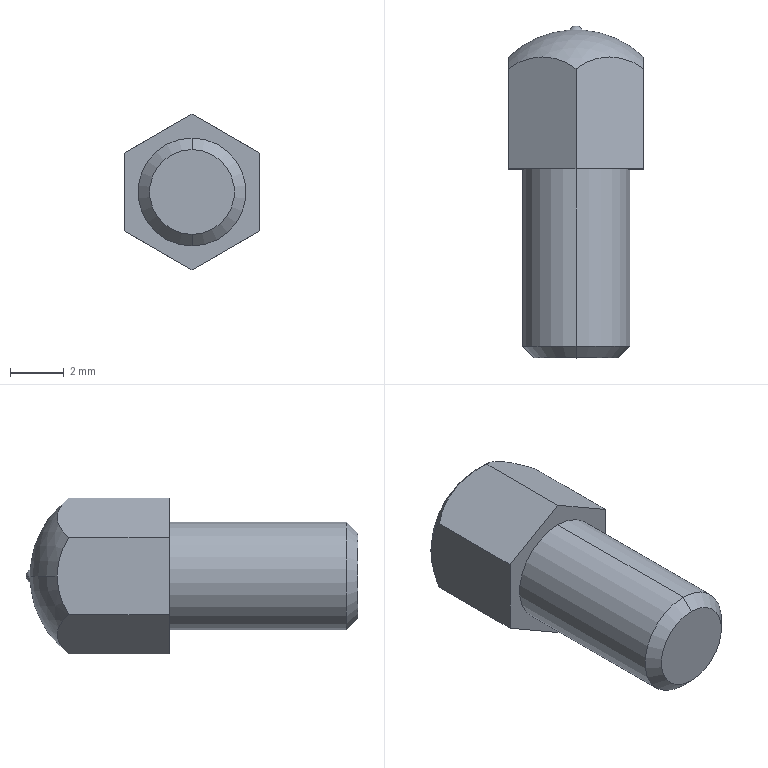Part | STEP file | HG15_34310002 | 1 solid | 16 faces | box 5 x 12.3 x 5.774 mm | volume 186.95 mm3 | plane 8 | sphere 4 | cone 2 | cylinder 2 | commonest cylinder face diameters 4 x2
STEP:
#1=CARTESIAN_POINT('',(0.,0.,0.));
#2=DIRECTION('',(0.,0.,1.));
#3=DIRECTION('',(1.,0.,0.));
#4=AXIS2_PLACEMENT_3D('',#1,#2,#3);
#5=CARTESIAN_POINT('',(-2.5,3.711,-1.443));
#6=VERTEX_POINT('',#5);
#7=CARTESIAN_POINT('',(-2.5,4.15,0.));
#8=VERTEX_POINT('',#7);
#9=CARTESIAN_POINT('',(-2.5,1.556,0.));
#10=DIRECTION('',(1.,0.,0.));
#11=DIRECTION('',(0.,0.,-1.));
#12=AXIS2_PLACEMENT_3D('',#9,#10,#11);
#13=CIRCLE('',#12,2.594);
#14=CARTESIAN_POINT('',(0.,1.556,0.));
#15=DIRECTION('',(0.,0.,-1.));
#16=DIRECTION('',(1.,0.,0.));
#17=AXIS2_PLACEMENT_3D('',#14,#15,#16);
#18=SPHERICAL_SURFACE('',#17,3.602);
#19=CARTESIAN_POINT('',(3.853,0.4122));
#20=CARTESIAN_POINT('',(3.856,0.4064));
#21=CARTESIAN_POINT('',(3.862,0.3947));
#22=CARTESIAN_POINT('',(3.87,0.3769));
#23=CARTESIAN_POINT('',(3.878,0.359));
#24=CARTESIAN_POINT('',(3.885,0.3409));
#25=CARTESIAN_POINT('',(3.892,0.3227));
#26=CARTESIAN_POINT('',(3.898,0.3043));
#27=CARTESIAN_POINT('',(3.904,0.2858));
#28=CARTESIAN_POINT('',(3.909,0.2673));
#29=CARTESIAN_POINT('',(3.914,0.2486));
#30=CARTESIAN_POINT('',(3.919,0.2298));
#31=CARTESIAN_POINT('',(3.923,0.211));
#32=CARTESIAN_POINT('',(3.927,0.192));
#33=CARTESIAN_POINT('',(3.931,0.173));
#34=CARTESIAN_POINT('',(3.934,0.1539));
#35=CARTESIAN_POINT('',(3.937,0.1348));
#36=CARTESIAN_POINT('',(3.939,0.1156));
#37=CARTESIAN_POINT('',(3.941,0.09643));
#38=CARTESIAN_POINT('',(3.943,0.07719));
#39=CARTESIAN_POINT('',(3.944,0.05791));
#40=CARTESIAN_POINT('',(3.945,0.03862));
#41=CARTESIAN_POINT('',(3.945,0.01931));
#42=CARTESIAN_POINT('',(3.945,0.006438));
#43=CARTESIAN_POINT('',(3.945,0.));
#44=B_SPLINE_CURVE_WITH_KNOTS('',3,(#19,#20,#21,#22,#23,#24,#25,#26,#27,#28,#29,#30,#31,#32,#33,#34,#35,#36,#37,#38,#39,#40,#41,#42,#43),.UNSPECIFIED.,.F.,.F.,(4,1,1,1,1,1,1,1,1,1,1,1,1,1,1,1,1,1,1,1,1,1,4),(0.9807,1.007,1.034,1.061,1.088,1.115,1.142,1.168,1.195,1.222,1.249,1.276,1.303,1.329,1.356,1.383,1.41,1.437,1.463,1.49,1.517,1.544,1.571),.QUASI_UNIFORM_KNOTS.);
#45=(GEOMETRIC_REPRESENTATION_CONTEXT(2)PARAMETRIC_REPRESENTATION_CONTEXT()REPRESENTATION_CONTEXT('',''));
#46=DEFINITIONAL_REPRESENTATION('',(#44),#45);
#47=PCURVE('',#18,#46);
#48=CARTESIAN_POINT('',(-2.5,5.3,-1.443));
#49=DIRECTION('',(1.,0.,0.));
#50=DIRECTION('',(0.,0.,-1.));
#51=AXIS2_PLACEMENT_3D('',#48,#49,#50);
#52=PLANE('',#51);
#53=CARTESIAN_POINT('',(-1.443,-3.744));
#54=DIRECTION('',(1.,0.));
#55=AXIS2_PLACEMENT_2D('',#53,#54);
#56=CIRCLE('',#55,2.594);
#57=(GEOMETRIC_REPRESENTATION_CONTEXT(2)PARAMETRIC_REPRESENTATION_CONTEXT()REPRESENTATION_CONTEXT('',''));
#58=DEFINITIONAL_REPRESENTATION('',(#56),#57);
#59=PCURVE('',#52,#58);
#60=SURFACE_CURVE('',#13,(#47,#59),.PCURVE_S1.);
#61=EDGE_CURVE('',#6,#8,#60,.T.);
#62=ORIENTED_EDGE('',*,*,#61,.T.);
#63=CARTESIAN_POINT('',(-0.25,5.15,0.));
#64=VERTEX_POINT('',#63);
#65=CARTESIAN_POINT('',(0.,1.556,0.));
#66=DIRECTION('',(0.,0.,-1.));
#67=DIRECTION('',(-1.,0.,0.));
#68=AXIS2_PLACEMENT_3D('',#65,#66,#67);
#69=CIRCLE('',#68,3.602);
#70=CARTESIAN_POINT('',(3.142,0.));
#71=DIRECTION('',(1.,0.));
#72=VECTOR('',#71,1.);
#73=LINE('',#70,#72);
#74=(GEOMETRIC_REPRESENTATION_CONTEXT(2)PARAMETRIC_REPRESENTATION_CONTEXT()REPRESENTATION_CONTEXT('',''));
#75=DEFINITIONAL_REPRESENTATION('',(#73),#74);
#76=PCURVE('',#18,#75);
#77=CARTESIAN_POINT('',(0.,1.556,0.));
#78=DIRECTION('',(0.,0.,-1.));
#79=DIRECTION('',(1.,0.,0.));
#80=AXIS2_PLACEMENT_3D('',#77,#78,#79);
#81=SPHERICAL_SURFACE('',#80,3.602);
#82=CARTESIAN_POINT('',(3.142,0.));
#83=DIRECTION('',(1.,0.));
#84=VECTOR('',#83,1.);
#85=LINE('',#82,#84);
#86=(GEOMETRIC_REPRESENTATION_CONTEXT(2)PARAMETRIC_REPRESENTATION_CONTEXT()REPRESENTATION_CONTEXT('',''));
#87=DEFINITIONAL_REPRESENTATION('',(#85),#86);
#88=PCURVE('',#81,#87);
#89=SURFACE_CURVE('',#69,(#76,#88),.PCURVE_S1.);
#90=EDGE_CURVE('',#8,#64,#89,.T.);
#91=ORIENTED_EDGE('',*,*,#90,.T.);
#92=CARTESIAN_POINT('',(0.25,5.15,0.));
#93=VERTEX_POINT('',#92);
#94=CARTESIAN_POINT('',(0.,5.15,0.));
#95=DIRECTION('',(0.,1.,0.));
#96=DIRECTION('',(0.,0.,1.));
#97=AXIS2_PLACEMENT_3D('',#94,#95,#96);
#98=CIRCLE('',#97,0.25);
#99=CARTESIAN_POINT('',(4.782,0.));
#100=CARTESIAN_POINT('',(4.782,0.003304));
#101=CARTESIAN_POINT('',(4.781,0.00991));
#102=CARTESIAN_POINT('',(4.779,0.01962));
#103=CARTESIAN_POINT('',(4.776,0.02893));
#104=CARTESIAN_POINT('',(4.771,0.03766));
#105=CARTESIAN_POINT('',(4.765,0.04562));
#106=CARTESIAN_POINT('',(4.758,0.05265));
#107=CARTESIAN_POINT('',(4.75,0.05861));
#108=CARTESIAN_POINT('',(4.741,0.06338));
#109=CARTESIAN_POINT('',(4.732,0.06686));
#110=CARTESIAN_POINT('',(4.722,0.06898));
#111=CARTESIAN_POINT('',(4.712,0.06969));
#112=CARTESIAN_POINT('',(4.702,0.06898));
#113=CARTESIAN_POINT('',(4.693,0.06686));
#114=CARTESIAN_POINT('',(4.683,0.06338));
#115=CARTESIAN_POINT('',(4.675,0.05861));
#116=CARTESIAN_POINT('',(4.667,0.05265));
#117=CARTESIAN_POINT('',(4.66,0.04562));
#118=CARTESIAN_POINT('',(4.654,0.03766));
#119=CARTESIAN_POINT('',(4.649,0.02893));
#120=CARTESIAN_POINT('',(4.646,0.01962));
#121=CARTESIAN_POINT('',(4.643,0.00991));
#122=CARTESIAN_POINT('',(4.643,0.003304));
#123=CARTESIAN_POINT('',(4.643,0.));
#124=B_SPLINE_CURVE_WITH_KNOTS('',3,(#99,#100,#101,#102,#103,#104,#105,#106,#107,#108,#109,#110,#111,#112,#113,#114,#115,#116,#117,#118,#119,#120,#121,#122,#123),.UNSPECIFIED.,.F.,.F.,(4,1,1,1,1,1,1,1,1,1,1,1,1,1,1,1,1,1,1,1,1,1,4),(1.571,1.714,1.856,1.999,2.142,2.285,2.428,2.57,2.713,2.856,2.999,3.142,3.284,3.427,3.57,3.713,3.856,3.998,4.141,4.284,4.427,4.57,4.712),.QUASI_UNIFORM_KNOTS.);
#125=(GEOMETRIC_REPRESENTATION_CONTEXT(2)PARAMETRIC_REPRESENTATION_CONTEXT()REPRESENTATION_CONTEXT('',''));
#126=DEFINITIONAL_REPRESENTATION('',(#124),#125);
#127=PCURVE('',#18,#126);
#128=CARTESIAN_POINT('',(0.,5.017,0.));
#129=DIRECTION('',(0.,0.,-1.));
#130=DIRECTION('',(1.,0.,0.));
#131=AXIS2_PLACEMENT_3D('',#128,#129,#130);
#132=SPHERICAL_SURFACE('',#131,0.2833);
#133=CARTESIAN_POINT('',(5.793,0.));
#134=CARTESIAN_POINT('',(5.793,0.04199));
#135=CARTESIAN_POINT('',(5.79,0.126));
#136=CARTESIAN_POINT('',(5.777,0.2514));
#137=CARTESIAN_POINT('',(5.755,0.3756));
#138=CARTESIAN_POINT('',(5.721,0.4978));
#139=CARTESIAN_POINT('',(5.672,0.6168));
#140=CARTESIAN_POINT('',(5.604,0.7312));
#141=CARTESIAN_POINT('',(5.51,0.8383));
#142=CARTESIAN_POINT('',(5.382,0.9345));
#143=CARTESIAN_POINT('',(5.207,1.014));
#144=CARTESIAN_POINT('',(4.98,1.068));
#145=CARTESIAN_POINT('',(4.712,1.087));
#146=CARTESIAN_POINT('',(4.445,1.068));
#147=CARTESIAN_POINT('',(4.218,1.014));
#148=CARTESIAN_POINT('',(4.043,0.9345));
#149=CARTESIAN_POINT('',(3.914,0.8383));
#150=CARTESIAN_POINT('',(3.821,0.7312));
#151=CARTESIAN_POINT('',(3.753,0.6168));
#152=CARTESIAN_POINT('',(3.704,0.4978));
#153=CARTESIAN_POINT('',(3.67,0.3756));
#154=CARTESIAN_POINT('',(3.647,0.2514));
#155=CARTESIAN_POINT('',(3.634,0.126));
#156=CARTESIAN_POINT('',(3.632,0.04199));
#157=CARTESIAN_POINT('',(3.632,0.));
#158=B_SPLINE_CURVE_WITH_KNOTS('',3,(#133,#134,#135,#136,#137,#138,#139,#140,#141,#142,#143,#144,#145,#146,#147,#148,#149,#150,#151,#152,#153,#154,#155,#156,#157),.UNSPECIFIED.,.F.,.F.,(4,1,1,1,1,1,1,1,1,1,1,1,1,1,1,1,1,1,1,1,1,1,4),(1.571,1.714,1.856,1.999,2.142,2.285,2.428,2.57,2.713,2.856,2.999,3.142,3.284,3.427,3.57,3.713,3.856,3.998,4.141,4.284,4.427,4.57,4.712),.QUASI_UNIFORM_KNOTS.);
#159=(GEOMETRIC_REPRESENTATION_CONTEXT(2)PARAMETRIC_REPRESENTATION_CONTEXT()REPRESENTATION_CONTEXT('',''));
#160=DEFINITIONAL_REPRESENTATION('',(#158),#159);
#161=PCURVE('',#132,#160);
#162=SURFACE_CURVE('',#98,(#127,#161),.PCURVE_S1.);
#163=EDGE_CURVE('',#93,#64,#162,.T.);
#164=ORIENTED_EDGE('',*,*,#163,.F.);
#165=CARTESIAN_POINT('',(2.5,4.15,0.));
#166=VERTEX_POINT('',#165);
#167=CARTESIAN_POINT('',(0.,1.556,0.));
#168=DIRECTION('',(0.,0.,1.));
#169=DIRECTION('',(1.,0.,0.));
#170=AXIS2_PLACEMENT_3D('',#167,#168,#169);
#171=CIRCLE('',#170,3.602);
#172=CARTESIAN_POINT('',(6.283,0.));
#173=DIRECTION('',(-1.,0.));
#174=VECTOR('',#173,1.);
#175=LINE('',#172,#174);
#176=(GEOMETRIC_REPRESENTATION_CONTEXT(2)PARAMETRIC_REPRESENTATION_CONTEXT()REPRESENTATION_CONTEXT('',''));
#177=DEFINITIONAL_REPRESENTATION('',(#175),#176);
#178=PCURVE('',#18,#177);
#179=CARTESIAN_POINT('',(6.283,0.));
#180=DIRECTION('',(-1.,0.));
#181=VECTOR('',#180,1.);
#182=LINE('',#179,#181);
#183=(GEOMETRIC_REPRESENTATION_CONTEXT(2)PARAMETRIC_REPRESENTATION_CONTEXT()REPRESENTATION_CONTEXT('',''));
#184=DEFINITIONAL_REPRESENTATION('',(#182),#183);
#185=PCURVE('',#81,#184);
#186=SURFACE_CURVE('',#171,(#178,#185),.PCURVE_S1.);
#187=EDGE_CURVE('',#166,#93,#186,.T.);
#188=ORIENTED_EDGE('',*,*,#187,.F.);
#189=CARTESIAN_POINT('',(2.5,3.711,-1.443));
#190=VERTEX_POINT('',#189);
#191=CARTESIAN_POINT('',(2.5,1.556,0.));
#192=DIRECTION('',(-1.,0.,0.));
#193=DIRECTION('',(0.,0.,1.));
#194=AXIS2_PLACEMENT_3D('',#191,#192,#193);
#195=CIRCLE('',#194,2.594);
#196=CARTESIAN_POINT('',(5.479,0.));
#197=CARTESIAN_POINT('',(5.479,0.006438));
#198=CARTESIAN_POINT('',(5.48,0.01931));
#199=CARTESIAN_POINT('',(5.48,0.03862));
#200=CARTESIAN_POINT('',(5.481,0.05791));
#201=CARTESIAN_POINT('',(5.482,0.07719));
#202=CARTESIAN_POINT('',(5.484,0.09643));
#203=CARTESIAN_POINT('',(5.486,0.1156));
#204=CARTESIAN_POINT('',(5.488,0.1348));
#205=CARTESIAN_POINT('',(5.491,0.1539));
#206=CARTESIAN_POINT('',(5.494,0.173));
#207=CARTESIAN_POINT('',(5.498,0.192));
#208=CARTESIAN_POINT('',(5.501,0.211));
#209=CARTESIAN_POINT('',(5.506,0.2298));
#210=CARTESIAN_POINT('',(5.51,0.2486));
#211=CARTESIAN_POINT('',(5.515,0.2673));
#212=CARTESIAN_POINT('',(5.521,0.2858));
#213=CARTESIAN_POINT('',(5.527,0.3043));
#214=CARTESIAN_POINT('',(5.533,0.3227));
#215=CARTESIAN_POINT('',(5.54,0.3409));
#216=CARTESIAN_POINT('',(5.547,0.359));
#217=CARTESIAN_POINT('',(5.555,0.3769));
#218=CARTESIAN_POINT('',(5.563,0.3947));
#219=CARTESIAN_POINT('',(5.569,0.4064));
#220=CARTESIAN_POINT('',(5.572,0.4122));
#221=B_SPLINE_CURVE_WITH_KNOTS('',3,(#196,#197,#198,#199,#200,#201,#202,#203,#204,#205,#206,#207,#208,#209,#210,#211,#212,#213,#214,#215,#216,#217,#218,#219,#220),.UNSPECIFIED.,.F.,.F.,(4,1,1,1,1,1,1,1,1,1,1,1,1,1,1,1,1,1,1,1,1,1,4),(1.571,1.598,1.624,1.651,1.678,1.705,1.732,1.759,1.785,1.812,1.839,1.866,1.893,1.92,1.946,1.973,2.,2.027,2.054,2.08,2.107,2.134,2.161),.QUASI_UNIFORM_KNOTS.);
#222=(GEOMETRIC_REPRESENTATION_CONTEXT(2)PARAMETRIC_REPRESENTATION_CONTEXT()REPRESENTATION_CONTEXT('',''));
#223=DEFINITIONAL_REPRESENTATION('',(#221),#222);
#224=PCURVE('',#18,#223);
#225=CARTESIAN_POINT('',(2.5,5.3,1.443));
#226=DIRECTION('',(-1.,0.,0.));
#227=DIRECTION('',(0.,0.,1.));
#228=AXIS2_PLACEMENT_3D('',#225,#226,#227);
#229=PLANE('',#228);
#230=CARTESIAN_POINT('',(-1.443,-3.744));
#231=DIRECTION('',(1.,0.));
#232=AXIS2_PLACEMENT_2D('',#230,#231);
#233=CIRCLE('',#232,2.594);
#234=(GEOMETRIC_REPRESENTATION_CONTEXT(2)PARAMETRIC_REPRESENTATION_CONTEXT()REPRESENTATION_CONTEXT('',''));
#235=DEFINITIONAL_REPRESENTATION('',(#233),#234);
#236=PCURVE('',#229,#235);
#237=SURFACE_CURVE('',#195,(#224,#236),.PCURVE_S1.);
#238=EDGE_CURVE('',#166,#190,#237,.T.);
#239=ORIENTED_EDGE('',*,*,#238,.T.);
#240=CARTESIAN_POINT('',(0.,3.711,-2.887));
#241=VERTEX_POINT('',#240);
#242=CARTESIAN_POINT('',(1.25,1.556,-2.165));
#243=DIRECTION('',(-0.5,0.,0.866));
#244=DIRECTION('',(0.866,0.,0.5));
#245=AXIS2_PLACEMENT_3D('',#242,#243,#244);
#246=CIRCLE('',#245,2.594);
#247=CARTESIAN_POINT('',(5.572,0.4122));
#248=CARTESIAN_POINT('',(5.559,0.4181));
#249=CARTESIAN_POINT('',(5.534,0.43));
#250=CARTESIAN_POINT('',(5.497,0.4486));
#251=CARTESIAN_POINT('',(5.46,0.468));
#252=CARTESIAN_POINT('',(5.422,0.488));
#253=CARTESIAN_POINT('',(5.385,0.5087));
#254=CARTESIAN_POINT('',(5.348,0.53));
#255=CARTESIAN_POINT('',(5.311,0.5518));
#256=CARTESIAN_POINT('',(5.274,0.5743));
#257=CARTESIAN_POINT('',(5.236,0.5973));
#258=CARTESIAN_POINT('',(5.199,0.6207));
#259=CARTESIAN_POINT('',(5.162,0.6447));
#260=CARTESIAN_POINT('',(5.124,0.6691));
#261=CARTESIAN_POINT('',(5.086,0.6939));
#262=CARTESIAN_POINT('',(5.047,0.719));
#263=CARTESIAN_POINT('',(5.008,0.7445));
#264=CARTESIAN_POINT('',(4.969,0.7703));
#265=CARTESIAN_POINT('',(4.928,0.7964));
#266=CARTESIAN_POINT('',(4.887,0.8228));
#267=CARTESIAN_POINT('',(4.845,0.8493));
#268=CARTESIAN_POINT('',(4.802,0.8759));
#269=CARTESIAN_POINT('',(4.758,0.9027));
#270=CARTESIAN_POINT('',(4.728,0.9206));
#271=CARTESIAN_POINT('',(4.712,0.9295));
#272=B_SPLINE_CURVE_WITH_KNOTS('',3,(#247,#248,#249,#250,#251,#252,#253,#254,#255,#256,#257,#258,#259,#260,#261,#262,#263,#264,#265,#266,#267,#268,#269,#270,#271),.UNSPECIFIED.,.F.,.F.,(4,1,1,1,1,1,1,1,1,1,1,1,1,1,1,1,1,1,1,1,1,1,4),(0.9807,1.034,1.088,1.142,1.195,1.249,1.303,1.356,1.41,1.463,1.517,1.571,1.624,1.678,1.732,1.785,1.839,1.893,1.946,2.,2.054,2.107,2.161),.QUASI_UNIFORM_KNOTS.);
#273=(GEOMETRIC_REPRESENTATION_CONTEXT(2)PARAMETRIC_REPRESENTATION_CONTEXT()REPRESENTATION_CONTEXT('',''));
#274=DEFINITIONAL_REPRESENTATION('',(#272),#273);
#275=PCURVE('',#18,#274);
#276=CARTESIAN_POINT('',(2.5,5.3,-1.443));
#277=DIRECTION('',(-0.5,0.,0.866));
#278=DIRECTION('',(0.866,0.,0.5));
#279=AXIS2_PLACEMENT_3D('',#276,#277,#278);
#280=PLANE('',#279);
#281=CARTESIAN_POINT('',(-1.443,-3.744));
#282=DIRECTION('',(1.,0.));
#283=AXIS2_PLACEMENT_2D('',#281,#282);
#284=CIRCLE('',#283,2.594);
#285=(GEOMETRIC_REPRESENTATION_CONTEXT(2)PARAMETRIC_REPRESENTATION_CONTEXT()REPRESENTATION_CONTEXT('',''));
#286=DEFINITIONAL_REPRESENTATION('',(#284),#285);
#287=PCURVE('',#280,#286);
#288=SURFACE_CURVE('',#246,(#275,#287),.PCURVE_S1.);
#289=EDGE_CURVE('',#190,#241,#288,.T.);
#290=ORIENTED_EDGE('',*,*,#289,.T.);
#291=CARTESIAN_POINT('',(-1.25,1.556,-2.165));
#292=DIRECTION('',(0.5,0.,0.866));
#293=DIRECTION('',(0.866,0.,-0.5));
#294=AXIS2_PLACEMENT_3D('',#291,#292,#293);
#295=CIRCLE('',#294,2.594);
#296=CARTESIAN_POINT('',(4.712,0.9295));
#297=CARTESIAN_POINT('',(4.697,0.9206));
#298=CARTESIAN_POINT('',(4.666,0.9027));
#299=CARTESIAN_POINT('',(4.622,0.8759));
#300=CARTESIAN_POINT('',(4.579,0.8493));
#301=CARTESIAN_POINT('',(4.537,0.8228));
#302=CARTESIAN_POINT('',(4.496,0.7964));
#303=CARTESIAN_POINT('',(4.456,0.7703));
#304=CARTESIAN_POINT('',(4.417,0.7445));
#305=CARTESIAN_POINT('',(4.378,0.719));
#306=CARTESIAN_POINT('',(4.339,0.6939));
#307=CARTESIAN_POINT('',(4.301,0.6691));
#308=CARTESIAN_POINT('',(4.263,0.6447));
#309=CARTESIAN_POINT('',(4.226,0.6207));
#310=CARTESIAN_POINT('',(4.188,0.5973));
#311=CARTESIAN_POINT('',(4.151,0.5743));
#312=CARTESIAN_POINT('',(4.114,0.5518));
#313=CARTESIAN_POINT('',(4.077,0.53));
#314=CARTESIAN_POINT('',(4.04,0.5087));
#315=CARTESIAN_POINT('',(4.002,0.488));
#316=CARTESIAN_POINT('',(3.965,0.468));
#317=CARTESIAN_POINT('',(3.928,0.4486));
#318=CARTESIAN_POINT('',(3.891,0.43));
#319=CARTESIAN_POINT('',(3.866,0.4181));
#320=CARTESIAN_POINT('',(3.853,0.4122));
#321=B_SPLINE_CURVE_WITH_KNOTS('',3,(#296,#297,#298,#299,#300,#301,#302,#303,#304,#305,#306,#307,#308,#309,#310,#311,#312,#313,#314,#315,#316,#317,#318,#319,#320),.UNSPECIFIED.,.F.,.F.,(4,1,1,1,1,1,1,1,1,1,1,1,1,1,1,1,1,1,1,1,1,1,4),(0.9807,1.034,1.088,1.142,1.195,1.249,1.303,1.356,1.41,1.463,1.517,1.571,1.624,1.678,1.732,1.785,1.839,1.893,1.946,2.,2.054,2.107,2.161),.QUASI_UNIFORM_KNOTS.);
#322=(GEOMETRIC_REPRESENTATION_CONTEXT(2)PARAMETRIC_REPRESENTATION_CONTEXT()REPRESENTATION_CONTEXT('',''));
#323=DEFINITIONAL_REPRESENTATION('',(#321),#322);
#324=PCURVE('',#18,#323);
#325=CARTESIAN_POINT('',(0.,5.3,-2.887));
#326=DIRECTION('',(0.5,0.,0.866));
#327=DIRECTION('',(0.866,0.,-0.5));
#328=AXIS2_PLACEMENT_3D('',#325,#326,#327);
#329=PLANE('',#328);
#330=CARTESIAN_POINT('',(-1.443,-3.744));
#331=DIRECTION('',(1.,0.));
#332=AXIS2_PLACEMENT_2D('',#330,#331);
#333=CIRCLE('',#332,2.594);
#334=(GEOMETRIC_REPRESENTATION_CONTEXT(2)PARAMETRIC_REPRESENTATION_CONTEXT()REPRESENTATION_CONTEXT('',''));
#335=DEFINITIONAL_REPRESENTATION('',(#333),#334);
#336=PCURVE('',#329,#335);
#337=SURFACE_CURVE('',#295,(#324,#336),.PCURVE_S1.);
#338=EDGE_CURVE('',#241,#6,#337,.T.);
#339=ORIENTED_EDGE('',*,*,#338,.T.);
#340=EDGE_LOOP('',(#62,#91,#164,#188,#239,#290,#339));
#341=FACE_BOUND('',#340,.T.);
#342=ADVANCED_FACE('',(#341),#18,.T.);
#343=ORIENTED_EDGE('',*,*,#163,.T.);
#344=CARTESIAN_POINT('',(0.,5.3,0.));
#345=VERTEX_POINT('',#344);
#346=CARTESIAN_POINT('',(0.,5.017,0.));
#347=DIRECTION('',(0.,0.,-1.));
#348=DIRECTION('',(-1.,0.,0.));
#349=AXIS2_PLACEMENT_3D('',#346,#347,#348);
#350=CIRCLE('',#349,0.2833);
#351=CARTESIAN_POINT('',(3.142,0.));
#352=DIRECTION('',(1.,0.));
#353=VECTOR('',#352,1.);
#354=LINE('',#351,#353);
#355=(GEOMETRIC_REPRESENTATION_CONTEXT(2)PARAMETRIC_REPRESENTATION_CONTEXT()REPRESENTATION_CONTEXT('',''));
#356=DEFINITIONAL_REPRESENTATION('',(#354),#355);
#357=PCURVE('',#132,#356);
#358=CARTESIAN_POINT('',(0.,5.017,0.));
#359=DIRECTION('',(0.,0.,-1.));
#360=DIRECTION('',(1.,0.,0.));
#361=AXIS2_PLACEMENT_3D('',#358,#359,#360);
#362=SPHERICAL_SURFACE('',#361,0.2833);
#363=CARTESIAN_POINT('',(3.142,0.));
#364=DIRECTION('',(1.,0.));
#365=VECTOR('',#364,1.);
#366=LINE('',#363,#365);
#367=(GEOMETRIC_REPRESENTATION_CONTEXT(2)PARAMETRIC_REPRESENTATION_CONTEXT()REPRESENTATION_CONTEXT('',''));
#368=DEFINITIONAL_REPRESENTATION('',(#366),#367);
#369=PCURVE('',#362,#368);
#370=SURFACE_CURVE('',#350,(#357,#369),.PCURVE_S1.);
#371=EDGE_CURVE('',#64,#345,#370,.T.);
#372=ORIENTED_EDGE('',*,*,#371,.T.);
#373=CARTESIAN_POINT('',(0.,5.017,0.));
#374=DIRECTION('',(0.,0.,1.));
#375=DIRECTION('',(1.,0.,0.));
#376=AXIS2_PLACEMENT_3D('',#373,#374,#375);
#377=CIRCLE('',#376,0.2833);
#378=CARTESIAN_POINT('',(6.283,0.));
#379=DIRECTION('',(-1.,0.));
#380=VECTOR('',#379,1.);
#381=LINE('',#378,#380);
#382=(GEOMETRIC_REPRESENTATION_CONTEXT(2)PARAMETRIC_REPRESENTATION_CONTEXT()REPRESENTATION_CONTEXT('',''));
#383=DEFINITIONAL_REPRESENTATION('',(#381),#382);
#384=PCURVE('',#132,#383);
#385=CARTESIAN_POINT('',(6.283,0.));
#386=DIRECTION('',(-1.,0.));
#387=VECTOR('',#386,1.);
#388=LINE('',#385,#387);
#389=(GEOMETRIC_REPRESENTATION_CONTEXT(2)PARAMETRIC_REPRESENTATION_CONTEXT()REPRESENTATION_CONTEXT('',''));
#390=DEFINITIONAL_REPRESENTATION('',(#388),#389);
#391=PCURVE('',#362,#390);
#392=SURFACE_CURVE('',#377,(#384,#391),.PCURVE_S1.);
#393=EDGE_CURVE('',#93,#345,#392,.T.);
#394=ORIENTED_EDGE('',*,*,#393,.F.);
#395=EDGE_LOOP('',(#343,#372,#394));
#396=FACE_BOUND('',#395,.T.);
#397=ADVANCED_FACE('',(#396),#132,.T.);
#398=CARTESIAN_POINT('',(0.,-7.,1.571));
#399=VERTEX_POINT('',#398);
#400=CARTESIAN_POINT('',(0.,-7.,-1.571));
#401=VERTEX_POINT('',#400);
#402=CARTESIAN_POINT('',(0.,-7.,0.));
#403=DIRECTION('',(0.,1.,0.));
#404=DIRECTION('',(0.,0.,1.));
#405=AXIS2_PLACEMENT_3D('',#402,#403,#404);
#406=CIRCLE('',#405,1.571);
#407=CARTESIAN_POINT('',(0.,-7.,0.));
#408=DIRECTION('',(0.,1.,0.));
#409=DIRECTION('',(0.,0.,1.));
#410=AXIS2_PLACEMENT_3D('',#407,#408,#409);
#411=CONICAL_SURFACE('',#410,1.571,0.7854);
#412=CARTESIAN_POINT('',(0.,0.));
#413=DIRECTION('',(1.,0.));
#414=VECTOR('',#413,1.);
#415=LINE('',#412,#414);
#416=(GEOMETRIC_REPRESENTATION_CONTEXT(2)PARAMETRIC_REPRESENTATION_CONTEXT()REPRESENTATION_CONTEXT('',''));
#417=DEFINITIONAL_REPRESENTATION('',(#415),#416);
#418=PCURVE('',#411,#417);
#419=CARTESIAN_POINT('',(1.571,-7.,0.));
#420=DIRECTION('',(0.,1.,0.));
#421=DIRECTION('',(0.,0.,1.));
#422=AXIS2_PLACEMENT_3D('',#419,#420,#421);
#423=PLANE('',#422);
#424=CARTESIAN_POINT('',(0.,-1.571));
#425=DIRECTION('',(1.,0.));
#426=AXIS2_PLACEMENT_2D('',#424,#425);
#427=CIRCLE('',#426,1.571);
#428=(GEOMETRIC_REPRESENTATION_CONTEXT(2)PARAMETRIC_REPRESENTATION_CONTEXT()REPRESENTATION_CONTEXT('',''));
#429=DEFINITIONAL_REPRESENTATION('',(#427),#428);
#430=PCURVE('',#423,#429);
#431=SURFACE_CURVE('',#406,(#418,#430),.PCURVE_S1.);
#432=EDGE_CURVE('',#399,#401,#431,.T.);
#433=ORIENTED_EDGE('',*,*,#432,.T.);
#434=CARTESIAN_POINT('',(0.,-6.571,-2.));
#435=VERTEX_POINT('',#434);
#436=CARTESIAN_POINT('',(0.,-7.,-1.571));
#437=DIRECTION('',(0.,0.7071,-0.7071));
#438=VECTOR('',#437,1.);
#439=LINE('',#436,#438);
#440=CARTESIAN_POINT('',(3.142,0.));
#441=DIRECTION('',(0.,1.));
#442=VECTOR('',#441,1.);
#443=LINE('',#440,#442);
#444=(GEOMETRIC_REPRESENTATION_CONTEXT(2)PARAMETRIC_REPRESENTATION_CONTEXT()REPRESENTATION_CONTEXT('',''));
#445=DEFINITIONAL_REPRESENTATION('',(#443),#444);
#446=PCURVE('',#411,#445);
#447=CARTESIAN_POINT('',(0.,-7.,0.));
#448=DIRECTION('',(0.,1.,0.));
#449=DIRECTION('',(0.,0.,1.));
#450=AXIS2_PLACEMENT_3D('',#447,#448,#449);
#451=CONICAL_SURFACE('',#450,1.571,0.7854);
#452=CARTESIAN_POINT('',(3.142,0.));
#453=DIRECTION('',(0.,1.));
#454=VECTOR('',#453,1.);
#455=LINE('',#452,#454);
#456=(GEOMETRIC_REPRESENTATION_CONTEXT(2)PARAMETRIC_REPRESENTATION_CONTEXT()REPRESENTATION_CONTEXT('',''));
#457=DEFINITIONAL_REPRESENTATION('',(#455),#456);
#458=PCURVE('',#451,#457);
#459=SURFACE_CURVE('',#439,(#446,#458),.PCURVE_S1.);
#460=EDGE_CURVE('',#401,#435,#459,.T.);
#461=ORIENTED_EDGE('',*,*,#460,.T.);
#462=CARTESIAN_POINT('',(0.,-6.571,2.));
#463=VERTEX_POINT('',#462);
#464=CARTESIAN_POINT('',(0.,-6.571,0.));
#465=DIRECTION('',(0.,1.,0.));
#466=DIRECTION('',(0.,0.,1.));
#467=AXIS2_PLACEMENT_3D('',#464,#465,#466);
#468=CIRCLE('',#467,2.);
#469=CARTESIAN_POINT('',(0.,0.4295));
#470=DIRECTION('',(1.,0.));
#471=VECTOR('',#470,1.);
#472=LINE('',#469,#471);
#473=(GEOMETRIC_REPRESENTATION_CONTEXT(2)PARAMETRIC_REPRESENTATION_CONTEXT()REPRESENTATION_CONTEXT('',''));
#474=DEFINITIONAL_REPRESENTATION('',(#472),#473);
#475=PCURVE('',#411,#474);
#476=CARTESIAN_POINT('',(0.,-7.,0.));
#477=DIRECTION('',(0.,1.,0.));
#478=DIRECTION('',(0.,0.,1.));
#479=AXIS2_PLACEMENT_3D('',#476,#477,#478);
#480=CYLINDRICAL_SURFACE('',#479,2.);
#481=CARTESIAN_POINT('',(0.,0.4295));
#482=DIRECTION('',(1.,0.));
#483=VECTOR('',#482,1.);
#484=LINE('',#481,#483);
#485=(GEOMETRIC_REPRESENTATION_CONTEXT(2)PARAMETRIC_REPRESENTATION_CONTEXT()REPRESENTATION_CONTEXT('',''));
#486=DEFINITIONAL_REPRESENTATION('',(#484),#485);
#487=PCURVE('',#480,#486);
#488=SURFACE_CURVE('',#468,(#475,#487),.PCURVE_S1.);
#489=EDGE_CURVE('',#463,#435,#488,.T.);
#490=ORIENTED_EDGE('',*,*,#489,.F.);
#491=CARTESIAN_POINT('',(0.,-7.,1.571));
#492=DIRECTION('',(0.,0.7071,0.7071));
#493=VECTOR('',#492,1.);
#494=LINE('',#491,#493);
#495=CARTESIAN_POINT('',(0.,0.));
#496=DIRECTION('',(0.,1.));
#497=VECTOR('',#496,1.);
#498=LINE('',#495,#497);
#499=(GEOMETRIC_REPRESENTATION_CONTEXT(2)PARAMETRIC_REPRESENTATION_CONTEXT()REPRESENTATION_CONTEXT('',''));
#500=DEFINITIONAL_REPRESENTATION('',(#498),#499);
#501=PCURVE('',#411,#500);
#502=CARTESIAN_POINT('',(6.283,0.));
#503=DIRECTION('',(0.,1.));
#504=VECTOR('',#503,1.);
#505=LINE('',#502,#504);
#506=(GEOMETRIC_REPRESENTATION_CONTEXT(2)PARAMETRIC_REPRESENTATION_CONTEXT()REPRESENTATION_CONTEXT('',''));
#507=DEFINITIONAL_REPRESENTATION('',(#505),#506);
#508=PCURVE('',#451,#507);
#509=SURFACE_CURVE('',#494,(#501,#508),.PCURVE_S1.);
#510=EDGE_CURVE('',#399,#463,#509,.T.);
#511=ORIENTED_EDGE('',*,*,#510,.F.);
#512=EDGE_LOOP('',(#433,#461,#490,#511));
#513=FACE_BOUND('',#512,.T.);
#514=ADVANCED_FACE('',(#513),#411,.T.);
#515=ORIENTED_EDGE('',*,*,#489,.T.);
#516=CARTESIAN_POINT('',(0.,0.,-2.));
#517=VERTEX_POINT('',#516);
#518=CARTESIAN_POINT('',(0.,-7.,-2.));
#519=DIRECTION('',(0.,1.,0.));
#520=VECTOR('',#519,1.);
#521=LINE('',#518,#520);
#522=CARTESIAN_POINT('',(3.142,0.));
#523=DIRECTION('',(0.,1.));
#524=VECTOR('',#523,1.);
#525=LINE('',#522,#524);
#526=(GEOMETRIC_REPRESENTATION_CONTEXT(2)PARAMETRIC_REPRESENTATION_CONTEXT()REPRESENTATION_CONTEXT('',''));
#527=DEFINITIONAL_REPRESENTATION('',(#525),#526);
#528=PCURVE('',#480,#527);
#529=CARTESIAN_POINT('',(0.,-7.,0.));
#530=DIRECTION('',(0.,1.,0.));
#531=DIRECTION('',(0.,0.,1.));
#532=AXIS2_PLACEMENT_3D('',#529,#530,#531);
#533=CYLINDRICAL_SURFACE('',#532,2.);
#534=CARTESIAN_POINT('',(3.142,0.));
#535=DIRECTION('',(0.,1.));
#536=VECTOR('',#535,1.);
#537=LINE('',#534,#536);
#538=(GEOMETRIC_REPRESENTATION_CONTEXT(2)PARAMETRIC_REPRESENTATION_CONTEXT()REPRESENTATION_CONTEXT('',''));
#539=DEFINITIONAL_REPRESENTATION('',(#537),#538);
#540=PCURVE('',#533,#539);
#541=SURFACE_CURVE('',#521,(#528,#540),.PCURVE_S1.);
#542=EDGE_CURVE('',#435,#517,#541,.T.);
#543=ORIENTED_EDGE('',*,*,#542,.T.);
#544=CARTESIAN_POINT('',(0.,0.,2.));
#545=VERTEX_POINT('',#544);
#546=CARTESIAN_POINT('',(0.,0.,0.));
#547=DIRECTION('',(0.,1.,0.));
#548=DIRECTION('',(0.,0.,1.));
#549=AXIS2_PLACEMENT_3D('',#546,#547,#548);
#550=CIRCLE('',#549,2.);
#551=CARTESIAN_POINT('',(0.,7.));
#552=DIRECTION('',(1.,0.));
#553=VECTOR('',#552,1.);
#554=LINE('',#551,#553);
#555=(GEOMETRIC_REPRESENTATION_CONTEXT(2)PARAMETRIC_REPRESENTATION_CONTEXT()REPRESENTATION_CONTEXT('',''));
#556=DEFINITIONAL_REPRESENTATION('',(#554),#555);
#557=PCURVE('',#480,#556);
#558=CARTESIAN_POINT('',(3.,0.,0.));
#559=DIRECTION('',(0.,1.,0.));
#560=DIRECTION('',(0.,0.,1.));
#561=AXIS2_PLACEMENT_3D('',#558,#559,#560);
#562=PLANE('',#561);
#563=CARTESIAN_POINT('',(0.,-3.));
#564=DIRECTION('',(1.,0.));
#565=AXIS2_PLACEMENT_2D('',#563,#564);
#566=CIRCLE('',#565,2.);
#567=(GEOMETRIC_REPRESENTATION_CONTEXT(2)PARAMETRIC_REPRESENTATION_CONTEXT()REPRESENTATION_CONTEXT('',''));
#568=DEFINITIONAL_REPRESENTATION('',(#566),#567);
#569=PCURVE('',#562,#568);
#570=SURFACE_CURVE('',#550,(#557,#569),.PCURVE_S1.);
#571=EDGE_CURVE('',#545,#517,#570,.T.);
#572=ORIENTED_EDGE('',*,*,#571,.F.);
#573=CARTESIAN_POINT('',(0.,-7.,2.));
#574=DIRECTION('',(0.,1.,0.));
#575=VECTOR('',#574,1.);
#576=LINE('',#573,#575);
#577=CARTESIAN_POINT('',(0.,0.));
#578=DIRECTION('',(0.,1.));
#579=VECTOR('',#578,1.);
#580=LINE('',#577,#579);
#581=(GEOMETRIC_REPRESENTATION_CONTEXT(2)PARAMETRIC_REPRESENTATION_CONTEXT()REPRESENTATION_CONTEXT('',''));
#582=DEFINITIONAL_REPRESENTATION('',(#580),#581);
#583=PCURVE('',#480,#582);
#584=CARTESIAN_POINT('',(6.283,0.));
#585=DIRECTION('',(0.,1.));
#586=VECTOR('',#585,1.);
#587=LINE('',#584,#586);
#588=(GEOMETRIC_REPRESENTATION_CONTEXT(2)PARAMETRIC_REPRESENTATION_CONTEXT()REPRESENTATION_CONTEXT('',''));
#589=DEFINITIONAL_REPRESENTATION('',(#587),#588);
#590=PCURVE('',#533,#589);
#591=SURFACE_CURVE('',#576,(#583,#590),.PCURVE_S1.);
#592=EDGE_CURVE('',#463,#545,#591,.T.);
#593=ORIENTED_EDGE('',*,*,#592,.F.);
#594=EDGE_LOOP('',(#515,#543,#572,#593));
#595=FACE_BOUND('',#594,.T.);
#596=ADVANCED_FACE('',(#595),#480,.T.);
#597=CARTESIAN_POINT('',(-2.5,0.,1.443));
#598=VERTEX_POINT('',#597);
#599=CARTESIAN_POINT('',(0.,0.,2.887));
#600=VERTEX_POINT('',#599);
#601=CARTESIAN_POINT('',(-2.5,0.,1.443));
#602=DIRECTION('',(0.866,0.,0.5));
#603=VECTOR('',#602,1.);
#604=LINE('',#601,#603);
#605=CARTESIAN_POINT('',(1.443,-5.5));
#606=DIRECTION('',(0.5,0.866));
#607=VECTOR('',#606,1.);
#608=LINE('',#605,#607);
#609=(GEOMETRIC_REPRESENTATION_CONTEXT(2)PARAMETRIC_REPRESENTATION_CONTEXT()REPRESENTATION_CONTEXT('',''));
#610=DEFINITIONAL_REPRESENTATION('',(#608),#609);
#611=PCURVE('',#562,#610);
#612=CARTESIAN_POINT('',(-2.5,5.3,1.443));
#613=DIRECTION('',(0.5,0.,-0.866));
#614=DIRECTION('',(-0.866,0.,-0.5));
#615=AXIS2_PLACEMENT_3D('',#612,#613,#614);
#616=PLANE('',#615);
#617=CARTESIAN_POINT('',(0.,-5.3));
#618=DIRECTION('',(-1.,0.));
#619=VECTOR('',#618,1.);
#620=LINE('',#617,#619);
#621=(GEOMETRIC_REPRESENTATION_CONTEXT(2)PARAMETRIC_REPRESENTATION_CONTEXT()REPRESENTATION_CONTEXT('',''));
#622=DEFINITIONAL_REPRESENTATION('',(#620),#621);
#623=PCURVE('',#616,#622);
#624=SURFACE_CURVE('',#604,(#611,#623),.PCURVE_S1.);
#625=EDGE_CURVE('',#598,#600,#624,.T.);
#626=ORIENTED_EDGE('',*,*,#625,.F.);
#627=CARTESIAN_POINT('',(-2.5,0.,-1.443));
#628=VERTEX_POINT('',#627);
#629=CARTESIAN_POINT('',(-2.5,0.,-1.443));
#630=DIRECTION('',(0.,0.,1.));
#631=VECTOR('',#630,1.);
#632=LINE('',#629,#631);
#633=CARTESIAN_POINT('',(-1.443,-5.5));
#634=DIRECTION('',(1.,0.));
#635=VECTOR('',#634,1.);
#636=LINE('',#633,#635);
#637=(GEOMETRIC_REPRESENTATION_CONTEXT(2)PARAMETRIC_REPRESENTATION_CONTEXT()REPRESENTATION_CONTEXT('',''));
#638=DEFINITIONAL_REPRESENTATION('',(#636),#637);
#639=PCURVE('',#562,#638);
#640=CARTESIAN_POINT('',(0.,-5.3));
#641=DIRECTION('',(-1.,0.));
#642=VECTOR('',#641,1.);
#643=LINE('',#640,#642);
#644=(GEOMETRIC_REPRESENTATION_CONTEXT(2)PARAMETRIC_REPRESENTATION_CONTEXT()REPRESENTATION_CONTEXT('',''));
#645=DEFINITIONAL_REPRESENTATION('',(#643),#644);
#646=PCURVE('',#52,#645);
#647=SURFACE_CURVE('',#632,(#639,#646),.PCURVE_S1.);
#648=EDGE_CURVE('',#628,#598,#647,.T.);
#649=ORIENTED_EDGE('',*,*,#648,.F.);
#650=CARTESIAN_POINT('',(0.,0.,-2.887));
#651=VERTEX_POINT('',#650);
#652=CARTESIAN_POINT('',(0.,0.,-2.887));
#653=DIRECTION('',(-0.866,0.,0.5));
#654=VECTOR('',#653,1.);
#655=LINE('',#652,#654);
#656=CARTESIAN_POINT('',(-2.887,-3.));
#657=DIRECTION('',(0.5,-0.866));
#658=VECTOR('',#657,1.);
#659=LINE('',#656,#658);
#660=(GEOMETRIC_REPRESENTATION_CONTEXT(2)PARAMETRIC_REPRESENTATION_CONTEXT()REPRESENTATION_CONTEXT('',''));
#661=DEFINITIONAL_REPRESENTATION('',(#659),#660);
#662=PCURVE('',#562,#661);
#663=CARTESIAN_POINT('',(0.,-5.3));
#664=DIRECTION('',(-1.,0.));
#665=VECTOR('',#664,1.);
#666=LINE('',#663,#665);
#667=(GEOMETRIC_REPRESENTATION_CONTEXT(2)PARAMETRIC_REPRESENTATION_CONTEXT()REPRESENTATION_CONTEXT('',''));
#668=DEFINITIONAL_REPRESENTATION('',(#666),#667);
#669=PCURVE('',#329,#668);
#670=SURFACE_CURVE('',#655,(#662,#669),.PCURVE_S1.);
#671=EDGE_CURVE('',#651,#628,#670,.T.);
#672=ORIENTED_EDGE('',*,*,#671,.F.);
#673=CARTESIAN_POINT('',(2.5,0.,-1.443));
#674=VERTEX_POINT('',#673);
#675=CARTESIAN_POINT('',(2.5,0.,-1.443));
#676=DIRECTION('',(-0.866,0.,-0.5));
#677=VECTOR('',#676,1.);
#678=LINE('',#675,#677);
#679=CARTESIAN_POINT('',(-1.443,-0.5));
#680=DIRECTION('',(-0.5,-0.866));
#681=VECTOR('',#680,1.);
#682=LINE('',#679,#681);
#683=(GEOMETRIC_REPRESENTATION_CONTEXT(2)PARAMETRIC_REPRESENTATION_CONTEXT()REPRESENTATION_CONTEXT('',''));
#684=DEFINITIONAL_REPRESENTATION('',(#682),#683);
#685=PCURVE('',#562,#684);
#686=CARTESIAN_POINT('',(0.,-5.3));
#687=DIRECTION('',(-1.,0.));
#688=VECTOR('',#687,1.);
#689=LINE('',#686,#688);
#690=(GEOMETRIC_REPRESENTATION_CONTEXT(2)PARAMETRIC_REPRESENTATION_CONTEXT()REPRESENTATION_CONTEXT('',''));
#691=DEFINITIONAL_REPRESENTATION('',(#689),#690);
#692=PCURVE('',#280,#691);
#693=SURFACE_CURVE('',#678,(#685,#692),.PCURVE_S1.);
#694=EDGE_CURVE('',#674,#651,#693,.T.);
#695=ORIENTED_EDGE('',*,*,#694,.F.);
#696=CARTESIAN_POINT('',(2.5,0.,1.443));
#697=VERTEX_POINT('',#696);
#698=CARTESIAN_POINT('',(2.5,0.,1.443));
#699=DIRECTION('',(0.,0.,-1.));
#700=VECTOR('',#699,1.);
#701=LINE('',#698,#700);
#702=CARTESIAN_POINT('',(1.443,-0.5));
#703=DIRECTION('',(-1.,0.));
#704=VECTOR('',#703,1.);
#705=LINE('',#702,#704);
#706=(GEOMETRIC_REPRESENTATION_CONTEXT(2)PARAMETRIC_REPRESENTATION_CONTEXT()REPRESENTATION_CONTEXT('',''));
#707=DEFINITIONAL_REPRESENTATION('',(#705),#706);
#708=PCURVE('',#562,#707);
#709=CARTESIAN_POINT('',(0.,-5.3));
#710=DIRECTION('',(-1.,0.));
#711=VECTOR('',#710,1.);
#712=LINE('',#709,#711);
#713=(GEOMETRIC_REPRESENTATION_CONTEXT(2)PARAMETRIC_REPRESENTATION_CONTEXT()REPRESENTATION_CONTEXT('',''));
#714=DEFINITIONAL_REPRESENTATION('',(#712),#713);
#715=PCURVE('',#229,#714);
#716=SURFACE_CURVE('',#701,(#708,#715),.PCURVE_S1.);
#717=EDGE_CURVE('',#697,#674,#716,.T.);
#718=ORIENTED_EDGE('',*,*,#717,.F.);
#719=CARTESIAN_POINT('',(0.,0.,2.887));
#720=DIRECTION('',(0.866,0.,-0.5));
#721=VECTOR('',#720,1.);
#722=LINE('',#719,#721);
#723=CARTESIAN_POINT('',(2.887,-3.));
#724=DIRECTION('',(-0.5,0.866));
#725=VECTOR('',#724,1.);
#726=LINE('',#723,#725);
#727=(GEOMETRIC_REPRESENTATION_CONTEXT(2)PARAMETRIC_REPRESENTATION_CONTEXT()REPRESENTATION_CONTEXT('',''));
#728=DEFINITIONAL_REPRESENTATION('',(#726),#727);
#729=PCURVE('',#562,#728);
#730=CARTESIAN_POINT('',(0.,5.3,2.887));
#731=DIRECTION('',(-0.5,0.,-0.866));
#732=DIRECTION('',(-0.866,0.,0.5));
#733=AXIS2_PLACEMENT_3D('',#730,#731,#732);
#734=PLANE('',#733);
#735=CARTESIAN_POINT('',(0.,-5.3));
#736=DIRECTION('',(-1.,0.));
#737=VECTOR('',#736,1.);
#738=LINE('',#735,#737);
#739=(GEOMETRIC_REPRESENTATION_CONTEXT(2)PARAMETRIC_REPRESENTATION_CONTEXT()REPRESENTATION_CONTEXT('',''));
#740=DEFINITIONAL_REPRESENTATION('',(#738),#739);
#741=PCURVE('',#734,#740);
#742=SURFACE_CURVE('',#722,(#729,#741),.PCURVE_S1.);
#743=EDGE_CURVE('',#600,#697,#742,.T.);
#744=ORIENTED_EDGE('',*,*,#743,.F.);
#745=EDGE_LOOP('',(#626,#649,#672,#695,#718,#744));
#746=FACE_BOUND('',#745,.T.);
#747=ORIENTED_EDGE('',*,*,#571,.T.);
#748=CARTESIAN_POINT('',(0.,0.,0.));
#749=DIRECTION('',(0.,1.,0.));
#750=DIRECTION('',(0.,0.,1.));
#751=AXIS2_PLACEMENT_3D('',#748,#749,#750);
#752=CIRCLE('',#751,2.);
#753=CARTESIAN_POINT('',(0.,-3.));
#754=DIRECTION('',(1.,0.));
#755=AXIS2_PLACEMENT_2D('',#753,#754);
#756=CIRCLE('',#755,2.);
#757=(GEOMETRIC_REPRESENTATION_CONTEXT(2)PARAMETRIC_REPRESENTATION_CONTEXT()REPRESENTATION_CONTEXT('',''));
#758=DEFINITIONAL_REPRESENTATION('',(#756),#757);
#759=PCURVE('',#562,#758);
#760=CARTESIAN_POINT('',(0.,7.));
#761=DIRECTION('',(1.,0.));
#762=VECTOR('',#761,1.);
#763=LINE('',#760,#762);
#764=(GEOMETRIC_REPRESENTATION_CONTEXT(2)PARAMETRIC_REPRESENTATION_CONTEXT()REPRESENTATION_CONTEXT('',''));
#765=DEFINITIONAL_REPRESENTATION('',(#763),#764);
#766=PCURVE('',#533,#765);
#767=SURFACE_CURVE('',#752,(#759,#766),.PCURVE_S1.);
#768=EDGE_CURVE('',#517,#545,#767,.T.);
#769=ORIENTED_EDGE('',*,*,#768,.T.);
#770=EDGE_LOOP('',(#747,#769));
#771=FACE_BOUND('',#770,.T.);
#772=ADVANCED_FACE('',(#746,#771),#562,.F.);
#773=ORIENTED_EDGE('',*,*,#542,.F.);
#774=CARTESIAN_POINT('',(0.,-6.571,0.));
#775=DIRECTION('',(0.,1.,0.));
#776=DIRECTION('',(0.,0.,1.));
#777=AXIS2_PLACEMENT_3D('',#774,#775,#776);
#778=CIRCLE('',#777,2.);
#779=CARTESIAN_POINT('',(0.,0.4295));
#780=DIRECTION('',(1.,0.));
#781=VECTOR('',#780,1.);
#782=LINE('',#779,#781);
#783=(GEOMETRIC_REPRESENTATION_CONTEXT(2)PARAMETRIC_REPRESENTATION_CONTEXT()REPRESENTATION_CONTEXT('',''));
#784=DEFINITIONAL_REPRESENTATION('',(#782),#783);
#785=PCURVE('',#533,#784);
#786=CARTESIAN_POINT('',(0.,0.4295));
#787=DIRECTION('',(1.,0.));
#788=VECTOR('',#787,1.);
#789=LINE('',#786,#788);
#790=(GEOMETRIC_REPRESENTATION_CONTEXT(2)PARAMETRIC_REPRESENTATION_CONTEXT()REPRESENTATION_CONTEXT('',''));
#791=DEFINITIONAL_REPRESENTATION('',(#789),#790);
#792=PCURVE('',#451,#791);
#793=SURFACE_CURVE('',#778,(#785,#792),.PCURVE_S1.);
#794=EDGE_CURVE('',#435,#463,#793,.T.);
#795=ORIENTED_EDGE('',*,*,#794,.T.);
#796=ORIENTED_EDGE('',*,*,#592,.T.);
#797=ORIENTED_EDGE('',*,*,#768,.F.);
#798=EDGE_LOOP('',(#773,#795,#796,#797));
#799=FACE_BOUND('',#798,.T.);
#800=ADVANCED_FACE('',(#799),#533,.T.);
#801=ORIENTED_EDGE('',*,*,#460,.F.);
#802=CARTESIAN_POINT('',(0.,-7.,0.));
#803=DIRECTION('',(0.,1.,0.));
#804=DIRECTION('',(0.,0.,1.));
#805=AXIS2_PLACEMENT_3D('',#802,#803,#804);
#806=CIRCLE('',#805,1.571);
#807=CARTESIAN_POINT('',(0.,0.));
#808=DIRECTION('',(1.,0.));
#809=VECTOR('',#808,1.);
#810=LINE('',#807,#809);
#811=(GEOMETRIC_REPRESENTATION_CONTEXT(2)PARAMETRIC_REPRESENTATION_CONTEXT()REPRESENTATION_CONTEXT('',''));
#812=DEFINITIONAL_REPRESENTATION('',(#810),#811);
#813=PCURVE('',#451,#812);
#814=CARTESIAN_POINT('',(0.,-1.571));
#815=DIRECTION('',(1.,0.));
#816=AXIS2_PLACEMENT_2D('',#814,#815);
#817=CIRCLE('',#816,1.571);
#818=(GEOMETRIC_REPRESENTATION_CONTEXT(2)PARAMETRIC_REPRESENTATION_CONTEXT()REPRESENTATION_CONTEXT('',''));
#819=DEFINITIONAL_REPRESENTATION('',(#817),#818);
#820=PCURVE('',#423,#819);
#821=SURFACE_CURVE('',#806,(#813,#820),.PCURVE_S1.);
#822=EDGE_CURVE('',#401,#399,#821,.T.);
#823=ORIENTED_EDGE('',*,*,#822,.T.);
#824=ORIENTED_EDGE('',*,*,#510,.T.);
#825=ORIENTED_EDGE('',*,*,#794,.F.);
#826=EDGE_LOOP('',(#801,#823,#824,#825));
#827=FACE_BOUND('',#826,.T.);
#828=ADVANCED_FACE('',(#827),#451,.T.);
#829=ORIENTED_EDGE('',*,*,#432,.F.);
#830=ORIENTED_EDGE('',*,*,#822,.F.);
#831=EDGE_LOOP('',(#829,#830));
#832=FACE_BOUND('',#831,.T.);
#833=ADVANCED_FACE('',(#832),#423,.F.);
#834=CARTESIAN_POINT('',(-2.5,5.3,-1.443));
#835=DIRECTION('',(0.,-1.,0.));
#836=VECTOR('',#835,1.);
#837=LINE('',#834,#836);
#838=CARTESIAN_POINT('',(0.,0.));
#839=DIRECTION('',(0.,-1.));
#840=VECTOR('',#839,1.);
#841=LINE('',#838,#840);
#842=(GEOMETRIC_REPRESENTATION_CONTEXT(2)PARAMETRIC_REPRESENTATION_CONTEXT()REPRESENTATION_CONTEXT('',''));
#843=DEFINITIONAL_REPRESENTATION('',(#841),#842);
#844=PCURVE('',#52,#843);
#845=CARTESIAN_POINT('',(-2.887,0.));
#846=DIRECTION('',(0.,-1.));
#847=VECTOR('',#846,1.);
#848=LINE('',#845,#847);
#849=(GEOMETRIC_REPRESENTATION_CONTEXT(2)PARAMETRIC_REPRESENTATION_CONTEXT()REPRESENTATION_CONTEXT('',''));
#850=DEFINITIONAL_REPRESENTATION('',(#848),#849);
#851=PCURVE('',#329,#850);
#852=SURFACE_CURVE('',#837,(#844,#851),.PCURVE_S1.);
#853=EDGE_CURVE('',#6,#628,#852,.T.);
#854=ORIENTED_EDGE('',*,*,#853,.T.);
#855=ORIENTED_EDGE('',*,*,#648,.T.);
#856=CARTESIAN_POINT('',(-2.5,3.711,1.443));
#857=VERTEX_POINT('',#856);
#858=CARTESIAN_POINT('',(-2.5,5.3,1.443));
#859=DIRECTION('',(0.,-1.,0.));
#860=VECTOR('',#859,1.);
#861=LINE('',#858,#860);
#862=CARTESIAN_POINT('',(-2.887,0.));
#863=DIRECTION('',(0.,-1.));
#864=VECTOR('',#863,1.);
#865=LINE('',#862,#864);
#866=(GEOMETRIC_REPRESENTATION_CONTEXT(2)PARAMETRIC_REPRESENTATION_CONTEXT()REPRESENTATION_CONTEXT('',''));
#867=DEFINITIONAL_REPRESENTATION('',(#865),#866);
#868=PCURVE('',#52,#867);
#869=CARTESIAN_POINT('',(0.,0.));
#870=DIRECTION('',(0.,-1.));
#871=VECTOR('',#870,1.);
#872=LINE('',#869,#871);
#873=(GEOMETRIC_REPRESENTATION_CONTEXT(2)PARAMETRIC_REPRESENTATION_CONTEXT()REPRESENTATION_CONTEXT('',''));
#874=DEFINITIONAL_REPRESENTATION('',(#872),#873);
#875=PCURVE('',#616,#874);
#876=SURFACE_CURVE('',#861,(#868,#875),.PCURVE_S1.);
#877=EDGE_CURVE('',#857,#598,#876,.T.);
#878=ORIENTED_EDGE('',*,*,#877,.F.);
#879=CARTESIAN_POINT('',(-2.5,1.556,0.));
#880=DIRECTION('',(1.,0.,0.));
#881=DIRECTION('',(0.,0.,-1.));
#882=AXIS2_PLACEMENT_3D('',#879,#880,#881);
#883=CIRCLE('',#882,2.594);
#884=CARTESIAN_POINT('',(-1.443,-3.744));
#885=DIRECTION('',(1.,0.));
#886=AXIS2_PLACEMENT_2D('',#884,#885);
#887=CIRCLE('',#886,2.594);
#888=(GEOMETRIC_REPRESENTATION_CONTEXT(2)PARAMETRIC_REPRESENTATION_CONTEXT()REPRESENTATION_CONTEXT('',''));
#889=DEFINITIONAL_REPRESENTATION('',(#887),#888);
#890=PCURVE('',#52,#889);
#891=CARTESIAN_POINT('',(3.945,0.));
#892=CARTESIAN_POINT('',(3.945,-0.006438));
#893=CARTESIAN_POINT('',(3.945,-0.01931));
#894=CARTESIAN_POINT('',(3.945,-0.03862));
#895=CARTESIAN_POINT('',(3.944,-0.05791));
#896=CARTESIAN_POINT('',(3.943,-0.07719));
#897=CARTESIAN_POINT('',(3.941,-0.09643));
#898=CARTESIAN_POINT('',(3.939,-0.1156));
#899=CARTESIAN_POINT('',(3.937,-0.1348));
#900=CARTESIAN_POINT('',(3.934,-0.1539));
#901=CARTESIAN_POINT('',(3.931,-0.173));
#902=CARTESIAN_POINT('',(3.927,-0.192));
#903=CARTESIAN_POINT('',(3.923,-0.211));
#904=CARTESIAN_POINT('',(3.919,-0.2298));
#905=CARTESIAN_POINT('',(3.914,-0.2486));
#906=CARTESIAN_POINT('',(3.909,-0.2673));
#907=CARTESIAN_POINT('',(3.904,-0.2858));
#908=CARTESIAN_POINT('',(3.898,-0.3043));
#909=CARTESIAN_POINT('',(3.892,-0.3227));
#910=CARTESIAN_POINT('',(3.885,-0.3409));
#911=CARTESIAN_POINT('',(3.878,-0.359));
#912=CARTESIAN_POINT('',(3.87,-0.3769));
#913=CARTESIAN_POINT('',(3.862,-0.3947));
#914=CARTESIAN_POINT('',(3.856,-0.4064));
#915=CARTESIAN_POINT('',(3.853,-0.4122));
#916=B_SPLINE_CURVE_WITH_KNOTS('',3,(#891,#892,#893,#894,#895,#896,#897,#898,#899,#900,#901,#902,#903,#904,#905,#906,#907,#908,#909,#910,#911,#912,#913,#914,#915),.UNSPECIFIED.,.F.,.F.,(4,1,1,1,1,1,1,1,1,1,1,1,1,1,1,1,1,1,1,1,1,1,4),(1.571,1.598,1.624,1.651,1.678,1.705,1.732,1.759,1.785,1.812,1.839,1.866,1.893,1.92,1.946,1.973,2.,2.027,2.054,2.08,2.107,2.134,2.161),.QUASI_UNIFORM_KNOTS.);
#917=(GEOMETRIC_REPRESENTATION_CONTEXT(2)PARAMETRIC_REPRESENTATION_CONTEXT()REPRESENTATION_CONTEXT('',''));
#918=DEFINITIONAL_REPRESENTATION('',(#916),#917);
#919=PCURVE('',#81,#918);
#920=SURFACE_CURVE('',#883,(#890,#919),.PCURVE_S1.);
#921=EDGE_CURVE('',#8,#857,#920,.T.);
#922=ORIENTED_EDGE('',*,*,#921,.F.);
#923=ORIENTED_EDGE('',*,*,#61,.F.);
#924=EDGE_LOOP('',(#854,#855,#878,#922,#923));
#925=FACE_BOUND('',#924,.T.);
#926=ADVANCED_FACE('',(#925),#52,.F.);
#927=ORIENTED_EDGE('',*,*,#877,.T.);
#928=ORIENTED_EDGE('',*,*,#625,.T.);
#929=CARTESIAN_POINT('',(0.,3.711,2.887));
#930=VERTEX_POINT('',#929);
#931=CARTESIAN_POINT('',(0.,5.3,2.887));
#932=DIRECTION('',(0.,-1.,0.));
#933=VECTOR('',#932,1.);
#934=LINE('',#931,#933);
#935=CARTESIAN_POINT('',(-2.887,0.));
#936=DIRECTION('',(0.,-1.));
#937=VECTOR('',#936,1.);
#938=LINE('',#935,#937);
#939=(GEOMETRIC_REPRESENTATION_CONTEXT(2)PARAMETRIC_REPRESENTATION_CONTEXT()REPRESENTATION_CONTEXT('',''));
#940=DEFINITIONAL_REPRESENTATION('',(#938),#939);
#941=PCURVE('',#616,#940);
#942=CARTESIAN_POINT('',(0.,0.));
#943=DIRECTION('',(0.,-1.));
#944=VECTOR('',#943,1.);
#945=LINE('',#942,#944);
#946=(GEOMETRIC_REPRESENTATION_CONTEXT(2)PARAMETRIC_REPRESENTATION_CONTEXT()REPRESENTATION_CONTEXT('',''));
#947=DEFINITIONAL_REPRESENTATION('',(#945),#946);
#948=PCURVE('',#734,#947);
#949=SURFACE_CURVE('',#934,(#941,#948),.PCURVE_S1.);
#950=EDGE_CURVE('',#930,#600,#949,.T.);
#951=ORIENTED_EDGE('',*,*,#950,.F.);
#952=CARTESIAN_POINT('',(-1.25,1.556,2.165));
#953=DIRECTION('',(0.5,0.,-0.866));
#954=DIRECTION('',(-0.866,0.,-0.5));
#955=AXIS2_PLACEMENT_3D('',#952,#953,#954);
#956=CIRCLE('',#955,2.594);
#957=CARTESIAN_POINT('',(-1.443,-3.744));
#958=DIRECTION('',(1.,0.));
#959=AXIS2_PLACEMENT_2D('',#957,#958);
#960=CIRCLE('',#959,2.594);
#961=(GEOMETRIC_REPRESENTATION_CONTEXT(2)PARAMETRIC_REPRESENTATION_CONTEXT()REPRESENTATION_CONTEXT('',''));
#962=DEFINITIONAL_REPRESENTATION('',(#960),#961);
#963=PCURVE('',#616,#962);
#964=CARTESIAN_POINT('',(3.853,-0.4122));
#965=CARTESIAN_POINT('',(3.866,-0.4181));
#966=CARTESIAN_POINT('',(3.891,-0.43));
#967=CARTESIAN_POINT('',(3.928,-0.4486));
#968=CARTESIAN_POINT('',(3.965,-0.468));
#969=CARTESIAN_POINT('',(4.002,-0.488));
#970=CARTESIAN_POINT('',(4.04,-0.5087));
#971=CARTESIAN_POINT('',(4.077,-0.53));
#972=CARTESIAN_POINT('',(4.114,-0.5518));
#973=CARTESIAN_POINT('',(4.151,-0.5743));
#974=CARTESIAN_POINT('',(4.188,-0.5973));
#975=CARTESIAN_POINT('',(4.226,-0.6207));
#976=CARTESIAN_POINT('',(4.263,-0.6447));
#977=CARTESIAN_POINT('',(4.301,-0.6691));
#978=CARTESIAN_POINT('',(4.339,-0.6939));
#979=CARTESIAN_POINT('',(4.378,-0.719));
#980=CARTESIAN_POINT('',(4.417,-0.7445));
#981=CARTESIAN_POINT('',(4.456,-0.7703));
#982=CARTESIAN_POINT('',(4.496,-0.7964));
#983=CARTESIAN_POINT('',(4.537,-0.8228));
#984=CARTESIAN_POINT('',(4.579,-0.8493));
#985=CARTESIAN_POINT('',(4.622,-0.8759));
#986=CARTESIAN_POINT('',(4.666,-0.9027));
#987=CARTESIAN_POINT('',(4.697,-0.9206));
#988=CARTESIAN_POINT('',(4.712,-0.9295));
#989=B_SPLINE_CURVE_WITH_KNOTS('',3,(#964,#965,#966,#967,#968,#969,#970,#971,#972,#973,#974,#975,#976,#977,#978,#979,#980,#981,#982,#983,#984,#985,#986,#987,#988),.UNSPECIFIED.,.F.,.F.,(4,1,1,1,1,1,1,1,1,1,1,1,1,1,1,1,1,1,1,1,1,1,4),(0.9807,1.034,1.088,1.142,1.195,1.249,1.303,1.356,1.41,1.463,1.517,1.571,1.624,1.678,1.732,1.785,1.839,1.893,1.946,2.,2.054,2.107,2.161),.QUASI_UNIFORM_KNOTS.);
#990=(GEOMETRIC_REPRESENTATION_CONTEXT(2)PARAMETRIC_REPRESENTATION_CONTEXT()REPRESENTATION_CONTEXT('',''));
#991=DEFINITIONAL_REPRESENTATION('',(#989),#990);
#992=PCURVE('',#81,#991);
#993=SURFACE_CURVE('',#956,(#963,#992),.PCURVE_S1.);
#994=EDGE_CURVE('',#857,#930,#993,.T.);
#995=ORIENTED_EDGE('',*,*,#994,.F.);
#996=EDGE_LOOP('',(#927,#928,#951,#995));
#997=FACE_BOUND('',#996,.T.);
#998=ADVANCED_FACE('',(#997),#616,.F.);
#999=ORIENTED_EDGE('',*,*,#950,.T.);
#1000=ORIENTED_EDGE('',*,*,#743,.T.);
#1001=CARTESIAN_POINT('',(2.5,3.711,1.443));
#1002=VERTEX_POINT('',#1001);
#1003=CARTESIAN_POINT('',(2.5,5.3,1.443));
#1004=DIRECTION('',(0.,-1.,0.));
#1005=VECTOR('',#1004,1.);
#1006=LINE('',#1003,#1005);
#1007=CARTESIAN_POINT('',(-2.887,0.));
#1008=DIRECTION('',(0.,-1.));
#1009=VECTOR('',#1008,1.);
#1010=LINE('',#1007,#1009);
#1011=(GEOMETRIC_REPRESENTATION_CONTEXT(2)PARAMETRIC_REPRESENTATION_CONTEXT()REPRESENTATION_CONTEXT('',''));
#1012=DEFINITIONAL_REPRESENTATION('',(#1010),#1011);
#1013=PCURVE('',#734,#1012);
#1014=CARTESIAN_POINT('',(0.,0.));
#1015=DIRECTION('',(0.,-1.));
#1016=VECTOR('',#1015,1.);
#1017=LINE('',#1014,#1016);
#1018=(GEOMETRIC_REPRESENTATION_CONTEXT(2)PARAMETRIC_REPRESENTATION_CONTEXT()REPRESENTATION_CONTEXT('',''));
#1019=DEFINITIONAL_REPRESENTATION('',(#1017),#1018);
#1020=PCURVE('',#229,#1019);
#1021=SURFACE_CURVE('',#1006,(#1013,#1020),.PCURVE_S1.);
#1022=EDGE_CURVE('',#1002,#697,#1021,.T.);
#1023=ORIENTED_EDGE('',*,*,#1022,.F.);
#1024=CARTESIAN_POINT('',(1.25,1.556,2.165));
#1025=DIRECTION('',(-0.5,0.,-0.866));
#1026=DIRECTION('',(-0.866,0.,0.5));
#1027=AXIS2_PLACEMENT_3D('',#1024,#1025,#1026);
#1028=CIRCLE('',#1027,2.594);
#1029=CARTESIAN_POINT('',(-1.443,-3.744));
#1030=DIRECTION('',(1.,0.));
#1031=AXIS2_PLACEMENT_2D('',#1029,#1030);
#1032=CIRCLE('',#1031,2.594);
#1033=(GEOMETRIC_REPRESENTATION_CONTEXT(2)PARAMETRIC_REPRESENTATION_CONTEXT()REPRESENTATION_CONTEXT('',''));
#1034=DEFINITIONAL_REPRESENTATION('',(#1032),#1033);
#1035=PCURVE('',#734,#1034);
#1036=CARTESIAN_POINT('',(4.712,-0.9295));
#1037=CARTESIAN_POINT('',(4.728,-0.9206));
#1038=CARTESIAN_POINT('',(4.758,-0.9027));
#1039=CARTESIAN_POINT('',(4.802,-0.8759));
#1040=CARTESIAN_POINT('',(4.845,-0.8493));
#1041=CARTESIAN_POINT('',(4.887,-0.8228));
#1042=CARTESIAN_POINT('',(4.928,-0.7964));
#1043=CARTESIAN_POINT('',(4.969,-0.7703));
#1044=CARTESIAN_POINT('',(5.008,-0.7445));
#1045=CARTESIAN_POINT('',(5.047,-0.719));
#1046=CARTESIAN_POINT('',(5.086,-0.6939));
#1047=CARTESIAN_POINT('',(5.124,-0.6691));
#1048=CARTESIAN_POINT('',(5.162,-0.6447));
#1049=CARTESIAN_POINT('',(5.199,-0.6207));
#1050=CARTESIAN_POINT('',(5.236,-0.5973));
#1051=CARTESIAN_POINT('',(5.274,-0.5743));
#1052=CARTESIAN_POINT('',(5.311,-0.5518));
#1053=CARTESIAN_POINT('',(5.348,-0.53));
#1054=CARTESIAN_POINT('',(5.385,-0.5087));
#1055=CARTESIAN_POINT('',(5.422,-0.488));
#1056=CARTESIAN_POINT('',(5.46,-0.468));
#1057=CARTESIAN_POINT('',(5.497,-0.4486));
#1058=CARTESIAN_POINT('',(5.534,-0.43));
#1059=CARTESIAN_POINT('',(5.559,-0.4181));
#1060=CARTESIAN_POINT('',(5.572,-0.4122));
#1061=B_SPLINE_CURVE_WITH_KNOTS('',3,(#1036,#1037,#1038,#1039,#1040,#1041,#1042,#1043,#1044,#1045,#1046,#1047,#1048,#1049,#1050,#1051,#1052,#1053,#1054,#1055,#1056,#1057,#1058,#1059,#1060),.UNSPECIFIED.,.F.,.F.,(4,1,1,1,1,1,1,1,1,1,1,1,1,1,1,1,1,1,1,1,1,1,4),(0.9807,1.034,1.088,1.142,1.195,1.249,1.303,1.356,1.41,1.463,1.517,1.571,1.624,1.678,1.732,1.785,1.839,1.893,1.946,2.,2.054,2.107,2.161),.QUASI_UNIFORM_KNOTS.);
#1062=(GEOMETRIC_REPRESENTATION_CONTEXT(2)PARAMETRIC_REPRESENTATION_CONTEXT()REPRESENTATION_CONTEXT('',''));
#1063=DEFINITIONAL_REPRESENTATION('',(#1061),#1062);
#1064=PCURVE('',#81,#1063);
#1065=SURFACE_CURVE('',#1028,(#1035,#1064),.PCURVE_S1.);
#1066=EDGE_CURVE('',#930,#1002,#1065,.T.);
#1067=ORIENTED_EDGE('',*,*,#1066,.F.);
#1068=EDGE_LOOP('',(#999,#1000,#1023,#1067));
#1069=FACE_BOUND('',#1068,.T.);
#1070=ADVANCED_FACE('',(#1069),#734,.F.);
#1071=ORIENTED_EDGE('',*,*,#1022,.T.);
#1072=ORIENTED_EDGE('',*,*,#717,.T.);
#1073=CARTESIAN_POINT('',(2.5,5.3,-1.443));
#1074=DIRECTION('',(0.,-1.,0.));
#1075=VECTOR('',#1074,1.);
#1076=LINE('',#1073,#1075);
#1077=CARTESIAN_POINT('',(-2.887,0.));
#1078=DIRECTION('',(0.,-1.));
#1079=VECTOR('',#1078,1.);
#1080=LINE('',#1077,#1079);
#1081=(GEOMETRIC_REPRESENTATION_CONTEXT(2)PARAMETRIC_REPRESENTATION_CONTEXT()REPRESENTATION_CONTEXT('',''));
#1082=DEFINITIONAL_REPRESENTATION('',(#1080),#1081);
#1083=PCURVE('',#229,#1082);
#1084=CARTESIAN_POINT('',(0.,0.));
#1085=DIRECTION('',(0.,-1.));
#1086=VECTOR('',#1085,1.);
#1087=LINE('',#1084,#1086);
#1088=(GEOMETRIC_REPRESENTATION_CONTEXT(2)PARAMETRIC_REPRESENTATION_CONTEXT()REPRESENTATION_CONTEXT('',''));
#1089=DEFINITIONAL_REPRESENTATION('',(#1087),#1088);
#1090=PCURVE('',#280,#1089);
#1091=SURFACE_CURVE('',#1076,(#1083,#1090),.PCURVE_S1.);
#1092=EDGE_CURVE('',#190,#674,#1091,.T.);
#1093=ORIENTED_EDGE('',*,*,#1092,.F.);
#1094=ORIENTED_EDGE('',*,*,#238,.F.);
#1095=CARTESIAN_POINT('',(2.5,1.556,0.));
#1096=DIRECTION('',(-1.,0.,0.));
#1097=DIRECTION('',(0.,0.,1.));
#1098=AXIS2_PLACEMENT_3D('',#1095,#1096,#1097);
#1099=CIRCLE('',#1098,2.594);
#1100=CARTESIAN_POINT('',(-1.443,-3.744));
#1101=DIRECTION('',(1.,0.));
#1102=AXIS2_PLACEMENT_2D('',#1100,#1101);
#1103=CIRCLE('',#1102,2.594);
#1104=(GEOMETRIC_REPRESENTATION_CONTEXT(2)PARAMETRIC_REPRESENTATION_CONTEXT()REPRESENTATION_CONTEXT('',''));
#1105=DEFINITIONAL_REPRESENTATION('',(#1103),#1104);
#1106=PCURVE('',#229,#1105);
#1107=CARTESIAN_POINT('',(5.572,-0.4122));
#1108=CARTESIAN_POINT('',(5.569,-0.4064));
#1109=CARTESIAN_POINT('',(5.563,-0.3947));
#1110=CARTESIAN_POINT('',(5.555,-0.3769));
#1111=CARTESIAN_POINT('',(5.547,-0.359));
#1112=CARTESIAN_POINT('',(5.54,-0.3409));
#1113=CARTESIAN_POINT('',(5.533,-0.3227));
#1114=CARTESIAN_POINT('',(5.527,-0.3043));
#1115=CARTESIAN_POINT('',(5.521,-0.2858));
#1116=CARTESIAN_POINT('',(5.515,-0.2673));
#1117=CARTESIAN_POINT('',(5.51,-0.2486));
#1118=CARTESIAN_POINT('',(5.506,-0.2298));
#1119=CARTESIAN_POINT('',(5.501,-0.211));
#1120=CARTESIAN_POINT('',(5.498,-0.192));
#1121=CARTESIAN_POINT('',(5.494,-0.173));
#1122=CARTESIAN_POINT('',(5.491,-0.1539));
#1123=CARTESIAN_POINT('',(5.488,-0.1348));
#1124=CARTESIAN_POINT('',(5.486,-0.1156));
#1125=CARTESIAN_POINT('',(5.484,-0.09643));
#1126=CARTESIAN_POINT('',(5.482,-0.07719));
#1127=CARTESIAN_POINT('',(5.481,-0.05791));
#1128=CARTESIAN_POINT('',(5.48,-0.03862));
#1129=CARTESIAN_POINT('',(5.48,-0.01931));
#1130=CARTESIAN_POINT('',(5.479,-0.006438));
#1131=CARTESIAN_POINT('',(5.479,0.));
#1132=B_SPLINE_CURVE_WITH_KNOTS('',3,(#1107,#1108,#1109,#1110,#1111,#1112,#1113,#1114,#1115,#1116,#1117,#1118,#1119,#1120,#1121,#1122,#1123,#1124,#1125,#1126,#1127,#1128,#1129,#1130,#1131),.UNSPECIFIED.,.F.,.F.,(4,1,1,1,1,1,1,1,1,1,1,1,1,1,1,1,1,1,1,1,1,1,4),(0.9807,1.007,1.034,1.061,1.088,1.115,1.142,1.168,1.195,1.222,1.249,1.276,1.303,1.329,1.356,1.383,1.41,1.437,1.463,1.49,1.517,1.544,1.571),.QUASI_UNIFORM_KNOTS.);
#1133=(GEOMETRIC_REPRESENTATION_CONTEXT(2)PARAMETRIC_REPRESENTATION_CONTEXT()REPRESENTATION_CONTEXT('',''));
#1134=DEFINITIONAL_REPRESENTATION('',(#1132),#1133);
#1135=PCURVE('',#81,#1134);
#1136=SURFACE_CURVE('',#1099,(#1106,#1135),.PCURVE_S1.);
#1137=EDGE_CURVE('',#1002,#166,#1136,.T.);
#1138=ORIENTED_EDGE('',*,*,#1137,.F.);
#1139=EDGE_LOOP('',(#1071,#1072,#1093,#1094,#1138));
#1140=FACE_BOUND('',#1139,.T.);
#1141=ADVANCED_FACE('',(#1140),#229,.F.);
#1142=ORIENTED_EDGE('',*,*,#1092,.T.);
#1143=ORIENTED_EDGE('',*,*,#694,.T.);
#1144=CARTESIAN_POINT('',(0.,5.3,-2.887));
#1145=DIRECTION('',(0.,-1.,0.));
#1146=VECTOR('',#1145,1.);
#1147=LINE('',#1144,#1146);
#1148=CARTESIAN_POINT('',(-2.887,0.));
#1149=DIRECTION('',(0.,-1.));
#1150=VECTOR('',#1149,1.);
#1151=LINE('',#1148,#1150);
#1152=(GEOMETRIC_REPRESENTATION_CONTEXT(2)PARAMETRIC_REPRESENTATION_CONTEXT()REPRESENTATION_CONTEXT('',''));
#1153=DEFINITIONAL_REPRESENTATION('',(#1151),#1152);
#1154=PCURVE('',#280,#1153);
#1155=CARTESIAN_POINT('',(0.,0.));
#1156=DIRECTION('',(0.,-1.));
#1157=VECTOR('',#1156,1.);
#1158=LINE('',#1155,#1157);
#1159=(GEOMETRIC_REPRESENTATION_CONTEXT(2)PARAMETRIC_REPRESENTATION_CONTEXT()REPRESENTATION_CONTEXT('',''));
#1160=DEFINITIONAL_REPRESENTATION('',(#1158),#1159);
#1161=PCURVE('',#329,#1160);
#1162=SURFACE_CURVE('',#1147,(#1154,#1161),.PCURVE_S1.);
#1163=EDGE_CURVE('',#241,#651,#1162,.T.);
#1164=ORIENTED_EDGE('',*,*,#1163,.F.);
#1165=ORIENTED_EDGE('',*,*,#289,.F.);
#1166=EDGE_LOOP('',(#1142,#1143,#1164,#1165));
#1167=FACE_BOUND('',#1166,.T.);
#1168=ADVANCED_FACE('',(#1167),#280,.F.);
#1169=ORIENTED_EDGE('',*,*,#1163,.T.);
#1170=ORIENTED_EDGE('',*,*,#671,.T.);
#1171=ORIENTED_EDGE('',*,*,#853,.F.);
#1172=ORIENTED_EDGE('',*,*,#338,.F.);
#1173=EDGE_LOOP('',(#1169,#1170,#1171,#1172));
#1174=FACE_BOUND('',#1173,.T.);
#1175=ADVANCED_FACE('',(#1174),#329,.F.);
#1176=ORIENTED_EDGE('',*,*,#371,.F.);
#1177=CARTESIAN_POINT('',(0.,5.15,0.));
#1178=DIRECTION('',(0.,1.,0.));
#1179=DIRECTION('',(0.,0.,1.));
#1180=AXIS2_PLACEMENT_3D('',#1177,#1178,#1179);
#1181=CIRCLE('',#1180,0.25);
#1182=CARTESIAN_POINT('',(3.632,0.));
#1183=CARTESIAN_POINT('',(3.632,-0.04199));
#1184=CARTESIAN_POINT('',(3.634,-0.126));
#1185=CARTESIAN_POINT('',(3.647,-0.2514));
#1186=CARTESIAN_POINT('',(3.67,-0.3756));
#1187=CARTESIAN_POINT('',(3.704,-0.4978));
#1188=CARTESIAN_POINT('',(3.753,-0.6168));
#1189=CARTESIAN_POINT('',(3.821,-0.7312));
#1190=CARTESIAN_POINT('',(3.914,-0.8383));
#1191=CARTESIAN_POINT('',(4.043,-0.9345));
#1192=CARTESIAN_POINT('',(4.218,-1.014));
#1193=CARTESIAN_POINT('',(4.445,-1.068));
#1194=CARTESIAN_POINT('',(4.712,-1.087));
#1195=CARTESIAN_POINT('',(4.98,-1.068));
#1196=CARTESIAN_POINT('',(5.207,-1.014));
#1197=CARTESIAN_POINT('',(5.382,-0.9345));
#1198=CARTESIAN_POINT('',(5.51,-0.8383));
#1199=CARTESIAN_POINT('',(5.604,-0.7312));
#1200=CARTESIAN_POINT('',(5.672,-0.6168));
#1201=CARTESIAN_POINT('',(5.721,-0.4978));
#1202=CARTESIAN_POINT('',(5.755,-0.3756));
#1203=CARTESIAN_POINT('',(5.777,-0.2514));
#1204=CARTESIAN_POINT('',(5.79,-0.126));
#1205=CARTESIAN_POINT('',(5.793,-0.04199));
#1206=CARTESIAN_POINT('',(5.793,0.));
#1207=B_SPLINE_CURVE_WITH_KNOTS('',3,(#1182,#1183,#1184,#1185,#1186,#1187,#1188,#1189,#1190,#1191,#1192,#1193,#1194,#1195,#1196,#1197,#1198,#1199,#1200,#1201,#1202,#1203,#1204,#1205,#1206),.UNSPECIFIED.,.F.,.F.,(4,1,1,1,1,1,1,1,1,1,1,1,1,1,1,1,1,1,1,1,1,1,4),(4.712,4.855,4.998,5.141,5.284,5.426,5.569,5.712,5.855,5.998,6.14,6.283,6.426,6.569,6.712,6.854,6.997,7.14,7.283,7.426,7.568,7.711,7.854),.QUASI_UNIFORM_KNOTS.);
#1208=(GEOMETRIC_REPRESENTATION_CONTEXT(2)PARAMETRIC_REPRESENTATION_CONTEXT()REPRESENTATION_CONTEXT('',''));
#1209=DEFINITIONAL_REPRESENTATION('',(#1207),#1208);
#1210=PCURVE('',#362,#1209);
#1211=CARTESIAN_POINT('',(4.643,0.));
#1212=CARTESIAN_POINT('',(4.643,-0.003304));
#1213=CARTESIAN_POINT('',(4.643,-0.00991));
#1214=CARTESIAN_POINT('',(4.646,-0.01962));
#1215=CARTESIAN_POINT('',(4.649,-0.02893));
#1216=CARTESIAN_POINT('',(4.654,-0.03766));
#1217=CARTESIAN_POINT('',(4.66,-0.04562));
#1218=CARTESIAN_POINT('',(4.667,-0.05265));
#1219=CARTESIAN_POINT('',(4.675,-0.05861));
#1220=CARTESIAN_POINT('',(4.683,-0.06338));
#1221=CARTESIAN_POINT('',(4.693,-0.06686));
#1222=CARTESIAN_POINT('',(4.702,-0.06898));
#1223=CARTESIAN_POINT('',(4.712,-0.06969));
#1224=CARTESIAN_POINT('',(4.722,-0.06898));
#1225=CARTESIAN_POINT('',(4.732,-0.06686));
#1226=CARTESIAN_POINT('',(4.741,-0.06338));
#1227=CARTESIAN_POINT('',(4.75,-0.05861));
#1228=CARTESIAN_POINT('',(4.758,-0.05265));
#1229=CARTESIAN_POINT('',(4.765,-0.04562));
#1230=CARTESIAN_POINT('',(4.771,-0.03766));
#1231=CARTESIAN_POINT('',(4.776,-0.02893));
#1232=CARTESIAN_POINT('',(4.779,-0.01962));
#1233=CARTESIAN_POINT('',(4.781,-0.00991));
#1234=CARTESIAN_POINT('',(4.782,-0.003304));
#1235=CARTESIAN_POINT('',(4.782,0.));
#1236=B_SPLINE_CURVE_WITH_KNOTS('',3,(#1211,#1212,#1213,#1214,#1215,#1216,#1217,#1218,#1219,#1220,#1221,#1222,#1223,#1224,#1225,#1226,#1227,#1228,#1229,#1230,#1231,#1232,#1233,#1234,#1235),.UNSPECIFIED.,.F.,.F.,(4,1,1,1,1,1,1,1,1,1,1,1,1,1,1,1,1,1,1,1,1,1,4),(4.712,4.855,4.998,5.141,5.284,5.426,5.569,5.712,5.855,5.998,6.14,6.283,6.426,6.569,6.712,6.854,6.997,7.14,7.283,7.426,7.568,7.711,7.854),.QUASI_UNIFORM_KNOTS.);
#1237=(GEOMETRIC_REPRESENTATION_CONTEXT(2)PARAMETRIC_REPRESENTATION_CONTEXT()REPRESENTATION_CONTEXT('',''));
#1238=DEFINITIONAL_REPRESENTATION('',(#1236),#1237);
#1239=PCURVE('',#81,#1238);
#1240=SURFACE_CURVE('',#1181,(#1210,#1239),.PCURVE_S1.);
#1241=EDGE_CURVE('',#64,#93,#1240,.T.);
#1242=ORIENTED_EDGE('',*,*,#1241,.T.);
#1243=ORIENTED_EDGE('',*,*,#393,.T.);
#1244=EDGE_LOOP('',(#1176,#1242,#1243));
#1245=FACE_BOUND('',#1244,.T.);
#1246=ADVANCED_FACE('',(#1245),#362,.T.);
#1247=ORIENTED_EDGE('',*,*,#90,.F.);
#1248=ORIENTED_EDGE('',*,*,#921,.T.);
#1249=ORIENTED_EDGE('',*,*,#994,.T.);
#1250=ORIENTED_EDGE('',*,*,#1066,.T.);
#1251=ORIENTED_EDGE('',*,*,#1137,.T.);
#1252=ORIENTED_EDGE('',*,*,#187,.T.);
#1253=ORIENTED_EDGE('',*,*,#1241,.F.);
#1254=EDGE_LOOP('',(#1247,#1248,#1249,#1250,#1251,#1252,#1253));
#1255=FACE_BOUND('',#1254,.T.);
#1256=ADVANCED_FACE('',(#1255),#81,.T.);
#1257=CLOSED_SHELL('',(#342,#397,#514,#596,#772,#800,#828,#833,#926,#998,#1070,#1141,#1168,#1175,#1246,#1256));
#1258=MANIFOLD_SOLID_BREP('',#1257);
#1259=(LENGTH_UNIT()NAMED_UNIT(*)SI_UNIT(.MILLI.,.METRE.));
#1260=UNCERTAINTY_MEASURE_WITH_UNIT(LENGTH_MEASURE(0.0000001),#1259,'','');
#1261=(NAMED_UNIT(*)PLANE_ANGLE_UNIT()SI_UNIT($,.RADIAN.));
#1262=(NAMED_UNIT(*)SI_UNIT($,.STERADIAN.)SOLID_ANGLE_UNIT());
#1263=(GEOMETRIC_REPRESENTATION_CONTEXT(3)GLOBAL_UNCERTAINTY_ASSIGNED_CONTEXT((#1260))GLOBAL_UNIT_ASSIGNED_CONTEXT((#1259,#1261,#1262))REPRESENTATION_CONTEXT('',''));
#1264=ADVANCED_BREP_SHAPE_REPRESENTATION('',(#4,#1258),#1263);